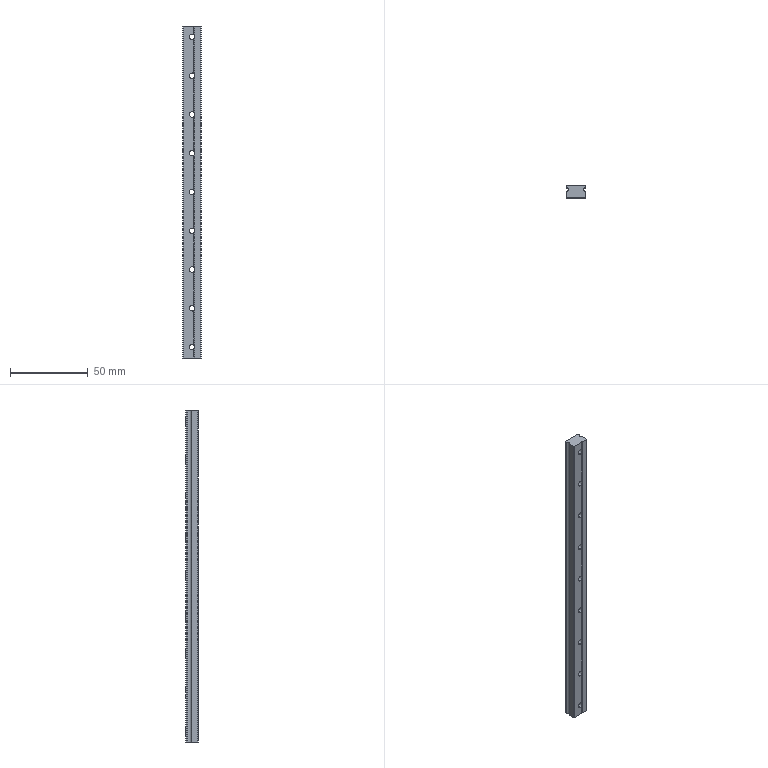Part | SolidWorks | features BaseBody 1, ICE 1, LPattern 1, MoveFace 1 | 1 solid | 62 faces | box 12 x 8 x 214 mm | volume 18147 mm3 | cylinder 40 | plane 22 | commonest cylinder face diameters 3.5 x18 6 x18 2.5 x3 0.6 x1